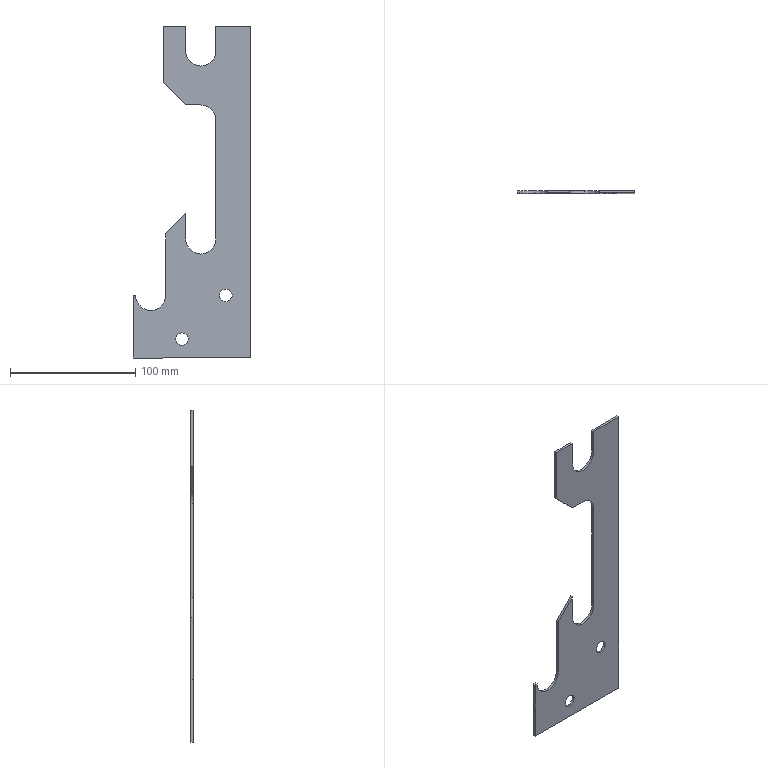Part | SolidWorks | features Extrusion 1 | 1 solid | 28 faces | box 94 x 2 x 265 mm | volume 27822 mm3 | plane 17 | cylinder 11 | commonest cylinder face diameters 24 x7 10 x4
STEP:
#1=CARTESIAN_POINT('',(74.,2.,-5.));
#2=VERTEX_POINT('',#1);
#3=CARTESIAN_POINT('',(74.,2.,5.));
#4=VERTEX_POINT('',#3);
#5=CARTESIAN_POINT('',(74.,2.,0.));
#6=DIRECTION('',(0.,1.,0.));
#7=DIRECTION('',(0.,0.,1.));
#8=AXIS2_PLACEMENT_3D('',#5,#6,#7);
#9=CIRCLE('',#8,5.);
#10=EDGE_CURVE('',#2,#4,#9,.T.);
#11=ORIENTED_EDGE('',*,*,#10,.T.);
#12=CARTESIAN_POINT('',(74.,0.,5.));
#13=VERTEX_POINT('',#12);
#14=CARTESIAN_POINT('',(74.,2.,5.));
#15=DIRECTION('',(0.,-1.,0.));
#16=VECTOR('',#15,1000.);
#17=LINE('',#14,#16);
#18=EDGE_CURVE('',#4,#13,#17,.T.);
#19=ORIENTED_EDGE('',*,*,#18,.T.);
#20=CARTESIAN_POINT('',(74.,0.,-5.));
#21=VERTEX_POINT('',#20);
#22=CARTESIAN_POINT('',(74.,0.,0.));
#23=DIRECTION('',(0.,1.,0.));
#24=DIRECTION('',(0.,0.,1.));
#25=AXIS2_PLACEMENT_3D('',#22,#23,#24);
#26=CIRCLE('',#25,5.);
#27=EDGE_CURVE('',#21,#13,#26,.T.);
#28=ORIENTED_EDGE('',*,*,#27,.F.);
#29=CARTESIAN_POINT('',(74.,2.,-5.));
#30=DIRECTION('',(0.,-1.,0.));
#31=VECTOR('',#30,1000.);
#32=LINE('',#29,#31);
#33=EDGE_CURVE('',#2,#21,#32,.T.);
#34=ORIENTED_EDGE('',*,*,#33,.F.);
#35=EDGE_LOOP('',(#11,#19,#28,#34));
#36=FACE_OUTER_BOUND('',#35,.T.);
#37=CARTESIAN_POINT('',(74.,2.,0.));
#38=DIRECTION('',(0.,-1.,0.));
#39=DIRECTION('',(0.,0.,-1.));
#40=AXIS2_PLACEMENT_3D('',#37,#38,#39);
#41=CYLINDRICAL_SURFACE('',#40,5.);
#42=ADVANCED_FACE('',(#36),#41,.F.);
#43=CARTESIAN_POINT('',(39.,2.,-40.));
#44=VERTEX_POINT('',#43);
#45=CARTESIAN_POINT('',(39.,2.,-30.));
#46=VERTEX_POINT('',#45);
#47=CARTESIAN_POINT('',(39.,2.,-35.));
#48=DIRECTION('',(0.,1.,0.));
#49=DIRECTION('',(0.,0.,1.));
#50=AXIS2_PLACEMENT_3D('',#47,#48,#49);
#51=CIRCLE('',#50,5.);
#52=EDGE_CURVE('',#44,#46,#51,.T.);
#53=ORIENTED_EDGE('',*,*,#52,.T.);
#54=CARTESIAN_POINT('',(39.,0.,-30.));
#55=VERTEX_POINT('',#54);
#56=CARTESIAN_POINT('',(39.,2.,-30.));
#57=DIRECTION('',(0.,-1.,0.));
#58=VECTOR('',#57,1000.);
#59=LINE('',#56,#58);
#60=EDGE_CURVE('',#46,#55,#59,.T.);
#61=ORIENTED_EDGE('',*,*,#60,.T.);
#62=CARTESIAN_POINT('',(39.,0.,-40.));
#63=VERTEX_POINT('',#62);
#64=CARTESIAN_POINT('',(39.,0.,-35.));
#65=DIRECTION('',(0.,1.,0.));
#66=DIRECTION('',(0.,0.,1.));
#67=AXIS2_PLACEMENT_3D('',#64,#65,#66);
#68=CIRCLE('',#67,5.);
#69=EDGE_CURVE('',#63,#55,#68,.T.);
#70=ORIENTED_EDGE('',*,*,#69,.F.);
#71=CARTESIAN_POINT('',(39.,2.,-40.));
#72=DIRECTION('',(0.,-1.,0.));
#73=VECTOR('',#72,1000.);
#74=LINE('',#71,#73);
#75=EDGE_CURVE('',#44,#63,#74,.T.);
#76=ORIENTED_EDGE('',*,*,#75,.F.);
#77=EDGE_LOOP('',(#53,#61,#70,#76));
#78=FACE_OUTER_BOUND('',#77,.T.);
#79=CARTESIAN_POINT('',(39.,2.,-35.));
#80=DIRECTION('',(0.,-1.,0.));
#81=DIRECTION('',(0.,0.,-1.));
#82=AXIS2_PLACEMENT_3D('',#79,#80,#81);
#83=CYLINDRICAL_SURFACE('',#82,5.);
#84=ADVANCED_FACE('',(#78),#83,.F.);
#85=CARTESIAN_POINT('',(54.,2.,183.));
#86=VERTEX_POINT('',#85);
#87=CARTESIAN_POINT('',(66.,2.,195.));
#88=VERTEX_POINT('',#87);
#89=CARTESIAN_POINT('',(54.,2.,195.));
#90=DIRECTION('',(0.,-1.,0.));
#91=DIRECTION('',(0.,0.,1.));
#92=AXIS2_PLACEMENT_3D('',#89,#90,#91);
#93=CIRCLE('',#92,12.);
#94=EDGE_CURVE('',#86,#88,#93,.T.);
#95=ORIENTED_EDGE('',*,*,#94,.F.);
#96=CARTESIAN_POINT('',(54.,0.,183.));
#97=VERTEX_POINT('',#96);
#98=CARTESIAN_POINT('',(54.,2.,183.));
#99=DIRECTION('',(0.,-1.,0.));
#100=VECTOR('',#99,1000.);
#101=LINE('',#98,#100);
#102=EDGE_CURVE('',#86,#97,#101,.T.);
#103=ORIENTED_EDGE('',*,*,#102,.T.);
#104=CARTESIAN_POINT('',(66.,0.,195.));
#105=VERTEX_POINT('',#104);
#106=CARTESIAN_POINT('',(54.,0.,195.));
#107=DIRECTION('',(0.,-1.,0.));
#108=DIRECTION('',(0.,0.,1.));
#109=AXIS2_PLACEMENT_3D('',#106,#107,#108);
#110=CIRCLE('',#109,12.);
#111=EDGE_CURVE('',#97,#105,#110,.T.);
#112=ORIENTED_EDGE('',*,*,#111,.T.);
#113=CARTESIAN_POINT('',(66.,2.,195.));
#114=DIRECTION('',(0.,-1.,0.));
#115=VECTOR('',#114,1000.);
#116=LINE('',#113,#115);
#117=EDGE_CURVE('',#88,#105,#116,.T.);
#118=ORIENTED_EDGE('',*,*,#117,.F.);
#119=EDGE_LOOP('',(#95,#103,#112,#118));
#120=FACE_OUTER_BOUND('',#119,.T.);
#121=CARTESIAN_POINT('',(54.,2.,195.));
#122=DIRECTION('',(0.,-1.,0.));
#123=DIRECTION('',(0.,0.,-1.));
#124=AXIS2_PLACEMENT_3D('',#121,#122,#123);
#125=CYLINDRICAL_SURFACE('',#124,12.);
#126=ADVANCED_FACE('',(#120),#125,.F.);
#127=CARTESIAN_POINT('',(54.,2.,33.));
#128=VERTEX_POINT('',#127);
#129=CARTESIAN_POINT('',(66.,2.,45.));
#130=VERTEX_POINT('',#129);
#131=CARTESIAN_POINT('',(54.,2.,45.));
#132=DIRECTION('',(0.,-1.,0.));
#133=DIRECTION('',(0.,0.,1.));
#134=AXIS2_PLACEMENT_3D('',#131,#132,#133);
#135=CIRCLE('',#134,12.);
#136=EDGE_CURVE('',#128,#130,#135,.T.);
#137=ORIENTED_EDGE('',*,*,#136,.F.);
#138=CARTESIAN_POINT('',(54.,0.,33.));
#139=VERTEX_POINT('',#138);
#140=CARTESIAN_POINT('',(54.,2.,33.));
#141=DIRECTION('',(0.,-1.,0.));
#142=VECTOR('',#141,1000.);
#143=LINE('',#140,#142);
#144=EDGE_CURVE('',#128,#139,#143,.T.);
#145=ORIENTED_EDGE('',*,*,#144,.T.);
#146=CARTESIAN_POINT('',(66.,0.,45.));
#147=VERTEX_POINT('',#146);
#148=CARTESIAN_POINT('',(54.,0.,45.));
#149=DIRECTION('',(0.,-1.,0.));
#150=DIRECTION('',(0.,0.,1.));
#151=AXIS2_PLACEMENT_3D('',#148,#149,#150);
#152=CIRCLE('',#151,12.);
#153=EDGE_CURVE('',#139,#147,#152,.T.);
#154=ORIENTED_EDGE('',*,*,#153,.T.);
#155=CARTESIAN_POINT('',(66.,2.,45.));
#156=DIRECTION('',(0.,-1.,0.));
#157=VECTOR('',#156,1000.);
#158=LINE('',#155,#157);
#159=EDGE_CURVE('',#130,#147,#158,.T.);
#160=ORIENTED_EDGE('',*,*,#159,.F.);
#161=EDGE_LOOP('',(#137,#145,#154,#160));
#162=FACE_OUTER_BOUND('',#161,.T.);
#163=CARTESIAN_POINT('',(54.,2.,45.));
#164=DIRECTION('',(0.,-1.,0.));
#165=DIRECTION('',(0.,0.,-1.));
#166=AXIS2_PLACEMENT_3D('',#163,#164,#165);
#167=CYLINDRICAL_SURFACE('',#166,12.);
#168=ADVANCED_FACE('',(#162),#167,.F.);
#169=CARTESIAN_POINT('',(14.,2.,-12.));
#170=VERTEX_POINT('',#169);
#171=CARTESIAN_POINT('',(26.,2.,0.));
#172=VERTEX_POINT('',#171);
#173=CARTESIAN_POINT('',(14.,2.,0.));
#174=DIRECTION('',(0.,-1.,0.));
#175=DIRECTION('',(0.,0.,1.));
#176=AXIS2_PLACEMENT_3D('',#173,#174,#175);
#177=CIRCLE('',#176,12.);
#178=EDGE_CURVE('',#170,#172,#177,.T.);
#179=ORIENTED_EDGE('',*,*,#178,.F.);
#180=CARTESIAN_POINT('',(14.,0.,-12.));
#181=VERTEX_POINT('',#180);
#182=CARTESIAN_POINT('',(14.,2.,-12.));
#183=DIRECTION('',(0.,-1.,0.));
#184=VECTOR('',#183,1000.);
#185=LINE('',#182,#184);
#186=EDGE_CURVE('',#170,#181,#185,.T.);
#187=ORIENTED_EDGE('',*,*,#186,.T.);
#188=CARTESIAN_POINT('',(26.,0.,0.));
#189=VERTEX_POINT('',#188);
#190=CARTESIAN_POINT('',(14.,0.,0.));
#191=DIRECTION('',(0.,-1.,0.));
#192=DIRECTION('',(0.,0.,1.));
#193=AXIS2_PLACEMENT_3D('',#190,#191,#192);
#194=CIRCLE('',#193,12.);
#195=EDGE_CURVE('',#181,#189,#194,.T.);
#196=ORIENTED_EDGE('',*,*,#195,.T.);
#197=CARTESIAN_POINT('',(26.,2.,0.));
#198=DIRECTION('',(0.,-1.,0.));
#199=VECTOR('',#198,1000.);
#200=LINE('',#197,#199);
#201=EDGE_CURVE('',#172,#189,#200,.T.);
#202=ORIENTED_EDGE('',*,*,#201,.F.);
#203=EDGE_LOOP('',(#179,#187,#196,#202));
#204=FACE_OUTER_BOUND('',#203,.T.);
#205=CARTESIAN_POINT('',(14.,2.,0.));
#206=DIRECTION('',(0.,-1.,0.));
#207=DIRECTION('',(0.,0.,-1.));
#208=AXIS2_PLACEMENT_3D('',#205,#206,#207);
#209=CYLINDRICAL_SURFACE('',#208,12.);
#210=ADVANCED_FACE('',(#204),#209,.F.);
#211=ORIENTED_EDGE('',*,*,#52,.F.);
#212=CARTESIAN_POINT('',(39.,2.,-35.));
#213=DIRECTION('',(0.,1.,0.));
#214=DIRECTION('',(0.,0.,1.));
#215=AXIS2_PLACEMENT_3D('',#212,#213,#214);
#216=CIRCLE('',#215,5.);
#217=EDGE_CURVE('',#46,#44,#216,.T.);
#218=ORIENTED_EDGE('',*,*,#217,.F.);
#219=EDGE_LOOP('',(#211,#218));
#220=FACE_BOUND('',#219,.T.);
#221=CARTESIAN_POINT('',(0.,2.,0.));
#222=VERTEX_POINT('',#221);
#223=CARTESIAN_POINT('',(2.,2.,0.));
#224=VERTEX_POINT('',#223);
#225=CARTESIAN_POINT('',(0.,2.,0.));
#226=DIRECTION('',(1.,0.,0.));
#227=VECTOR('',#226,1000.);
#228=LINE('',#225,#227);
#229=EDGE_CURVE('',#222,#224,#228,.T.);
#230=ORIENTED_EDGE('',*,*,#229,.T.);
#231=CARTESIAN_POINT('',(14.,2.,0.));
#232=DIRECTION('',(0.,-1.,0.));
#233=DIRECTION('',(0.,0.,1.));
#234=AXIS2_PLACEMENT_3D('',#231,#232,#233);
#235=CIRCLE('',#234,12.);
#236=EDGE_CURVE('',#224,#170,#235,.T.);
#237=ORIENTED_EDGE('',*,*,#236,.T.);
#238=ORIENTED_EDGE('',*,*,#178,.T.);
#239=CARTESIAN_POINT('',(26.,2.,49.));
#240=VERTEX_POINT('',#239);
#241=CARTESIAN_POINT('',(26.,2.,49.));
#242=DIRECTION('',(0.,0.,1.));
#243=VECTOR('',#242,1000.);
#244=LINE('',#241,#243);
#245=EDGE_CURVE('',#172,#240,#244,.T.);
#246=ORIENTED_EDGE('',*,*,#245,.T.);
#247=CARTESIAN_POINT('',(42.,2.,65.));
#248=VERTEX_POINT('',#247);
#249=CARTESIAN_POINT('',(42.,2.,65.));
#250=DIRECTION('',(0.7071,0.,0.7071));
#251=VECTOR('',#250,1000.);
#252=LINE('',#249,#251);
#253=EDGE_CURVE('',#240,#248,#252,.T.);
#254=ORIENTED_EDGE('',*,*,#253,.T.);
#255=CARTESIAN_POINT('',(42.,2.,45.));
#256=VERTEX_POINT('',#255);
#257=CARTESIAN_POINT('',(42.,2.,45.));
#258=DIRECTION('',(0.,0.,-1.));
#259=VECTOR('',#258,1000.);
#260=LINE('',#257,#259);
#261=EDGE_CURVE('',#248,#256,#260,.T.);
#262=ORIENTED_EDGE('',*,*,#261,.T.);
#263=CARTESIAN_POINT('',(54.,2.,45.));
#264=DIRECTION('',(0.,-1.,0.));
#265=DIRECTION('',(0.,0.,1.));
#266=AXIS2_PLACEMENT_3D('',#263,#264,#265);
#267=CIRCLE('',#266,12.);
#268=EDGE_CURVE('',#256,#128,#267,.T.);
#269=ORIENTED_EDGE('',*,*,#268,.T.);
#270=ORIENTED_EDGE('',*,*,#136,.T.);
#271=CARTESIAN_POINT('',(66.,2.,140.));
#272=VERTEX_POINT('',#271);
#273=CARTESIAN_POINT('',(66.,2.,45.));
#274=DIRECTION('',(0.,0.,1.));
#275=VECTOR('',#274,1000.);
#276=LINE('',#273,#275);
#277=EDGE_CURVE('',#130,#272,#276,.T.);
#278=ORIENTED_EDGE('',*,*,#277,.T.);
#279=CARTESIAN_POINT('',(54.,2.,152.));
#280=VERTEX_POINT('',#279);
#281=CARTESIAN_POINT('',(54.,2.,140.));
#282=DIRECTION('',(0.,-1.,0.));
#283=DIRECTION('',(0.,0.,-1.));
#284=AXIS2_PLACEMENT_3D('',#281,#282,#283);
#285=CIRCLE('',#284,12.);
#286=EDGE_CURVE('',#272,#280,#285,.T.);
#287=ORIENTED_EDGE('',*,*,#286,.T.);
#288=CARTESIAN_POINT('',(42.,2.,152.));
#289=VERTEX_POINT('',#288);
#290=CARTESIAN_POINT('',(54.,2.,152.));
#291=DIRECTION('',(-1.,0.,0.));
#292=VECTOR('',#291,1000.);
#293=LINE('',#290,#292);
#294=EDGE_CURVE('',#280,#289,#293,.T.);
#295=ORIENTED_EDGE('',*,*,#294,.T.);
#296=CARTESIAN_POINT('',(24.,2.,170.));
#297=VERTEX_POINT('',#296);
#298=CARTESIAN_POINT('',(42.,2.,152.));
#299=DIRECTION('',(-0.7071,0.,0.7071));
#300=VECTOR('',#299,1000.);
#301=LINE('',#298,#300);
#302=EDGE_CURVE('',#289,#297,#301,.T.);
#303=ORIENTED_EDGE('',*,*,#302,.T.);
#304=CARTESIAN_POINT('',(24.,2.,215.));
#305=VERTEX_POINT('',#304);
#306=CARTESIAN_POINT('',(24.,2.,170.));
#307=DIRECTION('',(0.,0.,1.));
#308=VECTOR('',#307,1000.);
#309=LINE('',#306,#308);
#310=EDGE_CURVE('',#297,#305,#309,.T.);
#311=ORIENTED_EDGE('',*,*,#310,.T.);
#312=CARTESIAN_POINT('',(42.,2.,215.));
#313=VERTEX_POINT('',#312);
#314=CARTESIAN_POINT('',(24.,2.,215.));
#315=DIRECTION('',(1.,0.,0.));
#316=VECTOR('',#315,1000.);
#317=LINE('',#314,#316);
#318=EDGE_CURVE('',#305,#313,#317,.T.);
#319=ORIENTED_EDGE('',*,*,#318,.T.);
#320=CARTESIAN_POINT('',(42.,2.,195.));
#321=VERTEX_POINT('',#320);
#322=CARTESIAN_POINT('',(42.,2.,215.));
#323=DIRECTION('',(0.,0.,-1.));
#324=VECTOR('',#323,1000.);
#325=LINE('',#322,#324);
#326=EDGE_CURVE('',#313,#321,#325,.T.);
#327=ORIENTED_EDGE('',*,*,#326,.T.);
#328=CARTESIAN_POINT('',(54.,2.,195.));
#329=DIRECTION('',(0.,-1.,0.));
#330=DIRECTION('',(0.,0.,1.));
#331=AXIS2_PLACEMENT_3D('',#328,#329,#330);
#332=CIRCLE('',#331,12.);
#333=EDGE_CURVE('',#321,#86,#332,.T.);
#334=ORIENTED_EDGE('',*,*,#333,.T.);
#335=ORIENTED_EDGE('',*,*,#94,.T.);
#336=CARTESIAN_POINT('',(66.,2.,215.));
#337=VERTEX_POINT('',#336);
#338=CARTESIAN_POINT('',(66.,2.,195.));
#339=DIRECTION('',(0.,0.,1.));
#340=VECTOR('',#339,1000.);
#341=LINE('',#338,#340);
#342=EDGE_CURVE('',#88,#337,#341,.T.);
#343=ORIENTED_EDGE('',*,*,#342,.T.);
#344=CARTESIAN_POINT('',(94.,2.,215.));
#345=VERTEX_POINT('',#344);
#346=CARTESIAN_POINT('',(94.,2.,215.));
#347=DIRECTION('',(1.,0.,0.));
#348=VECTOR('',#347,1000.);
#349=LINE('',#346,#348);
#350=EDGE_CURVE('',#337,#345,#349,.T.);
#351=ORIENTED_EDGE('',*,*,#350,.T.);
#352=CARTESIAN_POINT('',(94.,2.,-50.));
#353=VERTEX_POINT('',#352);
#354=CARTESIAN_POINT('',(94.,2.,-50.));
#355=DIRECTION('',(0.,0.,-1.));
#356=VECTOR('',#355,1000.);
#357=LINE('',#354,#356);
#358=EDGE_CURVE('',#345,#353,#357,.T.);
#359=ORIENTED_EDGE('',*,*,#358,.T.);
#360=CARTESIAN_POINT('',(0.,2.,-50.));
#361=VERTEX_POINT('',#360);
#362=CARTESIAN_POINT('',(0.,2.,-50.));
#363=DIRECTION('',(-1.,0.,0.));
#364=VECTOR('',#363,1000.);
#365=LINE('',#362,#364);
#366=EDGE_CURVE('',#353,#361,#365,.T.);
#367=ORIENTED_EDGE('',*,*,#366,.T.);
#368=CARTESIAN_POINT('',(0.,2.,0.));
#369=DIRECTION('',(0.,0.,1.));
#370=VECTOR('',#369,1000.);
#371=LINE('',#368,#370);
#372=EDGE_CURVE('',#361,#222,#371,.T.);
#373=ORIENTED_EDGE('',*,*,#372,.T.);
#374=EDGE_LOOP('',(#230,#237,#238,#246,#254,#262,#269,#270,#278,#287,#295,#303,#311,#319,#327,#334,#335,#343,#351,#359,#367,#373));
#375=FACE_OUTER_BOUND('',#374,.T.);
#376=ORIENTED_EDGE('',*,*,#10,.F.);
#377=CARTESIAN_POINT('',(74.,2.,0.));
#378=DIRECTION('',(0.,1.,0.));
#379=DIRECTION('',(0.,0.,1.));
#380=AXIS2_PLACEMENT_3D('',#377,#378,#379);
#381=CIRCLE('',#380,5.);
#382=EDGE_CURVE('',#4,#2,#381,.T.);
#383=ORIENTED_EDGE('',*,*,#382,.F.);
#384=EDGE_LOOP('',(#376,#383));
#385=FACE_BOUND('',#384,.T.);
#386=CARTESIAN_POINT('',(14.,2.,0.));
#387=DIRECTION('',(0.,1.,0.));
#388=DIRECTION('',(0.,0.,1.));
#389=AXIS2_PLACEMENT_3D('',#386,#387,#388);
#390=PLANE('',#389);
#391=ADVANCED_FACE('',(#220,#375,#385),#390,.T.);
#392=CARTESIAN_POINT('',(0.,0.,0.));
#393=VERTEX_POINT('',#392);
#394=CARTESIAN_POINT('',(2.,0.,0.));
#395=VERTEX_POINT('',#394);
#396=CARTESIAN_POINT('',(0.,0.,0.));
#397=DIRECTION('',(1.,0.,0.));
#398=VECTOR('',#397,1000.);
#399=LINE('',#396,#398);
#400=EDGE_CURVE('',#393,#395,#399,.T.);
#401=ORIENTED_EDGE('',*,*,#400,.F.);
#402=CARTESIAN_POINT('',(0.,0.,-50.));
#403=VERTEX_POINT('',#402);
#404=CARTESIAN_POINT('',(0.,0.,0.));
#405=DIRECTION('',(0.,0.,1.));
#406=VECTOR('',#405,1000.);
#407=LINE('',#404,#406);
#408=EDGE_CURVE('',#403,#393,#407,.T.);
#409=ORIENTED_EDGE('',*,*,#408,.F.);
#410=CARTESIAN_POINT('',(94.,0.,-50.));
#411=VERTEX_POINT('',#410);
#412=CARTESIAN_POINT('',(0.,0.,-50.));
#413=DIRECTION('',(-1.,0.,0.));
#414=VECTOR('',#413,1000.);
#415=LINE('',#412,#414);
#416=EDGE_CURVE('',#411,#403,#415,.T.);
#417=ORIENTED_EDGE('',*,*,#416,.F.);
#418=CARTESIAN_POINT('',(94.,0.,215.));
#419=VERTEX_POINT('',#418);
#420=CARTESIAN_POINT('',(94.,0.,-50.));
#421=DIRECTION('',(0.,0.,-1.));
#422=VECTOR('',#421,1000.);
#423=LINE('',#420,#422);
#424=EDGE_CURVE('',#419,#411,#423,.T.);
#425=ORIENTED_EDGE('',*,*,#424,.F.);
#426=CARTESIAN_POINT('',(66.,0.,215.));
#427=VERTEX_POINT('',#426);
#428=CARTESIAN_POINT('',(94.,0.,215.));
#429=DIRECTION('',(1.,0.,0.));
#430=VECTOR('',#429,1000.);
#431=LINE('',#428,#430);
#432=EDGE_CURVE('',#427,#419,#431,.T.);
#433=ORIENTED_EDGE('',*,*,#432,.F.);
#434=CARTESIAN_POINT('',(66.,0.,195.));
#435=DIRECTION('',(0.,0.,1.));
#436=VECTOR('',#435,1000.);
#437=LINE('',#434,#436);
#438=EDGE_CURVE('',#105,#427,#437,.T.);
#439=ORIENTED_EDGE('',*,*,#438,.F.);
#440=ORIENTED_EDGE('',*,*,#111,.F.);
#441=CARTESIAN_POINT('',(42.,0.,195.));
#442=VERTEX_POINT('',#441);
#443=CARTESIAN_POINT('',(54.,0.,195.));
#444=DIRECTION('',(0.,-1.,0.));
#445=DIRECTION('',(0.,0.,1.));
#446=AXIS2_PLACEMENT_3D('',#443,#444,#445);
#447=CIRCLE('',#446,12.);
#448=EDGE_CURVE('',#442,#97,#447,.T.);
#449=ORIENTED_EDGE('',*,*,#448,.F.);
#450=CARTESIAN_POINT('',(42.,0.,215.));
#451=VERTEX_POINT('',#450);
#452=CARTESIAN_POINT('',(42.,0.,215.));
#453=DIRECTION('',(0.,0.,-1.));
#454=VECTOR('',#453,1000.);
#455=LINE('',#452,#454);
#456=EDGE_CURVE('',#451,#442,#455,.T.);
#457=ORIENTED_EDGE('',*,*,#456,.F.);
#458=CARTESIAN_POINT('',(24.,0.,215.));
#459=VERTEX_POINT('',#458);
#460=CARTESIAN_POINT('',(24.,0.,215.));
#461=DIRECTION('',(1.,0.,0.));
#462=VECTOR('',#461,1000.);
#463=LINE('',#460,#462);
#464=EDGE_CURVE('',#459,#451,#463,.T.);
#465=ORIENTED_EDGE('',*,*,#464,.F.);
#466=CARTESIAN_POINT('',(24.,0.,170.));
#467=VERTEX_POINT('',#466);
#468=CARTESIAN_POINT('',(24.,0.,170.));
#469=DIRECTION('',(0.,0.,1.));
#470=VECTOR('',#469,1000.);
#471=LINE('',#468,#470);
#472=EDGE_CURVE('',#467,#459,#471,.T.);
#473=ORIENTED_EDGE('',*,*,#472,.F.);
#474=CARTESIAN_POINT('',(42.,0.,152.));
#475=VERTEX_POINT('',#474);
#476=CARTESIAN_POINT('',(42.,0.,152.));
#477=DIRECTION('',(-0.7071,0.,0.7071));
#478=VECTOR('',#477,1000.);
#479=LINE('',#476,#478);
#480=EDGE_CURVE('',#475,#467,#479,.T.);
#481=ORIENTED_EDGE('',*,*,#480,.F.);
#482=CARTESIAN_POINT('',(54.,0.,152.));
#483=VERTEX_POINT('',#482);
#484=CARTESIAN_POINT('',(54.,0.,152.));
#485=DIRECTION('',(-1.,0.,0.));
#486=VECTOR('',#485,1000.);
#487=LINE('',#484,#486);
#488=EDGE_CURVE('',#483,#475,#487,.T.);
#489=ORIENTED_EDGE('',*,*,#488,.F.);
#490=CARTESIAN_POINT('',(66.,0.,140.));
#491=VERTEX_POINT('',#490);
#492=CARTESIAN_POINT('',(54.,0.,140.));
#493=DIRECTION('',(0.,-1.,0.));
#494=DIRECTION('',(0.,0.,-1.));
#495=AXIS2_PLACEMENT_3D('',#492,#493,#494);
#496=CIRCLE('',#495,12.);
#497=EDGE_CURVE('',#491,#483,#496,.T.);
#498=ORIENTED_EDGE('',*,*,#497,.F.);
#499=CARTESIAN_POINT('',(66.,0.,45.));
#500=DIRECTION('',(0.,0.,1.));
#501=VECTOR('',#500,1000.);
#502=LINE('',#499,#501);
#503=EDGE_CURVE('',#147,#491,#502,.T.);
#504=ORIENTED_EDGE('',*,*,#503,.F.);
#505=ORIENTED_EDGE('',*,*,#153,.F.);
#506=CARTESIAN_POINT('',(42.,0.,45.));
#507=VERTEX_POINT('',#506);
#508=CARTESIAN_POINT('',(54.,0.,45.));
#509=DIRECTION('',(0.,-1.,0.));
#510=DIRECTION('',(0.,0.,1.));
#511=AXIS2_PLACEMENT_3D('',#508,#509,#510);
#512=CIRCLE('',#511,12.);
#513=EDGE_CURVE('',#507,#139,#512,.T.);
#514=ORIENTED_EDGE('',*,*,#513,.F.);
#515=CARTESIAN_POINT('',(42.,0.,65.));
#516=VERTEX_POINT('',#515);
#517=CARTESIAN_POINT('',(42.,0.,45.));
#518=DIRECTION('',(0.,0.,-1.));
#519=VECTOR('',#518,1000.);
#520=LINE('',#517,#519);
#521=EDGE_CURVE('',#516,#507,#520,.T.);
#522=ORIENTED_EDGE('',*,*,#521,.F.);
#523=CARTESIAN_POINT('',(26.,0.,49.));
#524=VERTEX_POINT('',#523);
#525=CARTESIAN_POINT('',(42.,0.,65.));
#526=DIRECTION('',(0.7071,0.,0.7071));
#527=VECTOR('',#526,1000.);
#528=LINE('',#525,#527);
#529=EDGE_CURVE('',#524,#516,#528,.T.);
#530=ORIENTED_EDGE('',*,*,#529,.F.);
#531=CARTESIAN_POINT('',(26.,0.,49.));
#532=DIRECTION('',(0.,0.,1.));
#533=VECTOR('',#532,1000.);
#534=LINE('',#531,#533);
#535=EDGE_CURVE('',#189,#524,#534,.T.);
#536=ORIENTED_EDGE('',*,*,#535,.F.);
#537=ORIENTED_EDGE('',*,*,#195,.F.);
#538=CARTESIAN_POINT('',(14.,0.,0.));
#539=DIRECTION('',(0.,-1.,0.));
#540=DIRECTION('',(0.,0.,1.));
#541=AXIS2_PLACEMENT_3D('',#538,#539,#540);
#542=CIRCLE('',#541,12.);
#543=EDGE_CURVE('',#395,#181,#542,.T.);
#544=ORIENTED_EDGE('',*,*,#543,.F.);
#545=EDGE_LOOP('',(#401,#409,#417,#425,#433,#439,#440,#449,#457,#465,#473,#481,#489,#498,#504,#505,#514,#522,#530,#536,#537,#544));
#546=FACE_OUTER_BOUND('',#545,.T.);
#547=ORIENTED_EDGE('',*,*,#69,.T.);
#548=CARTESIAN_POINT('',(39.,0.,-35.));
#549=DIRECTION('',(0.,1.,0.));
#550=DIRECTION('',(0.,0.,1.));
#551=AXIS2_PLACEMENT_3D('',#548,#549,#550);
#552=CIRCLE('',#551,5.);
#553=EDGE_CURVE('',#55,#63,#552,.T.);
#554=ORIENTED_EDGE('',*,*,#553,.T.);
#555=EDGE_LOOP('',(#547,#554));
#556=FACE_BOUND('',#555,.T.);
#557=ORIENTED_EDGE('',*,*,#27,.T.);
#558=CARTESIAN_POINT('',(74.,0.,0.));
#559=DIRECTION('',(0.,1.,0.));
#560=DIRECTION('',(0.,0.,1.));
#561=AXIS2_PLACEMENT_3D('',#558,#559,#560);
#562=CIRCLE('',#561,5.);
#563=EDGE_CURVE('',#13,#21,#562,.T.);
#564=ORIENTED_EDGE('',*,*,#563,.T.);
#565=EDGE_LOOP('',(#557,#564));
#566=FACE_BOUND('',#565,.T.);
#567=CARTESIAN_POINT('',(14.,0.,0.));
#568=DIRECTION('',(0.,1.,0.));
#569=DIRECTION('',(0.,0.,1.));
#570=AXIS2_PLACEMENT_3D('',#567,#568,#569);
#571=PLANE('',#570);
#572=ADVANCED_FACE('',(#546,#556,#566),#571,.F.);
#573=ORIENTED_EDGE('',*,*,#400,.T.);
#574=CARTESIAN_POINT('',(2.,2.,0.));
#575=DIRECTION('',(0.,-1.,0.));
#576=VECTOR('',#575,1000.);
#577=LINE('',#574,#576);
#578=EDGE_CURVE('',#224,#395,#577,.T.);
#579=ORIENTED_EDGE('',*,*,#578,.F.);
#580=ORIENTED_EDGE('',*,*,#229,.F.);
#581=CARTESIAN_POINT('',(0.,2.,0.));
#582=DIRECTION('',(0.,-1.,0.));
#583=VECTOR('',#582,1000.);
#584=LINE('',#581,#583);
#585=EDGE_CURVE('',#222,#393,#584,.T.);
#586=ORIENTED_EDGE('',*,*,#585,.T.);
#587=EDGE_LOOP('',(#573,#579,#580,#586));
#588=FACE_OUTER_BOUND('',#587,.T.);
#589=CARTESIAN_POINT('',(0.,2.,0.));
#590=DIRECTION('',(0.,0.,-1.));
#591=DIRECTION('',(-1.,0.,0.));
#592=AXIS2_PLACEMENT_3D('',#589,#590,#591);
#593=PLANE('',#592);
#594=ADVANCED_FACE('',(#588),#593,.F.);
#595=ORIENTED_EDGE('',*,*,#186,.F.);
#596=ORIENTED_EDGE('',*,*,#236,.F.);
#597=ORIENTED_EDGE('',*,*,#578,.T.);
#598=ORIENTED_EDGE('',*,*,#543,.T.);
#599=EDGE_LOOP('',(#595,#596,#597,#598));
#600=FACE_OUTER_BOUND('',#599,.T.);
#601=CARTESIAN_POINT('',(14.,2.,0.));
#602=DIRECTION('',(0.,-1.,0.));
#603=DIRECTION('',(0.,0.,-1.));
#604=AXIS2_PLACEMENT_3D('',#601,#602,#603);
#605=CYLINDRICAL_SURFACE('',#604,12.);
#606=ADVANCED_FACE('',(#600),#605,.F.);
#607=ORIENTED_EDGE('',*,*,#535,.T.);
#608=CARTESIAN_POINT('',(26.,2.,49.));
#609=DIRECTION('',(0.,-1.,0.));
#610=VECTOR('',#609,1000.);
#611=LINE('',#608,#610);
#612=EDGE_CURVE('',#240,#524,#611,.T.);
#613=ORIENTED_EDGE('',*,*,#612,.F.);
#614=ORIENTED_EDGE('',*,*,#245,.F.);
#615=ORIENTED_EDGE('',*,*,#201,.T.);
#616=EDGE_LOOP('',(#607,#613,#614,#615));
#617=FACE_OUTER_BOUND('',#616,.T.);
#618=CARTESIAN_POINT('',(26.,2.,49.));
#619=DIRECTION('',(1.,0.,0.));
#620=DIRECTION('',(0.,0.,-1.));
#621=AXIS2_PLACEMENT_3D('',#618,#619,#620);
#622=PLANE('',#621);
#623=ADVANCED_FACE('',(#617),#622,.F.);
#624=ORIENTED_EDGE('',*,*,#529,.T.);
#625=CARTESIAN_POINT('',(42.,2.,65.));
#626=DIRECTION('',(0.,-1.,0.));
#627=VECTOR('',#626,1000.);
#628=LINE('',#625,#627);
#629=EDGE_CURVE('',#248,#516,#628,.T.);
#630=ORIENTED_EDGE('',*,*,#629,.F.);
#631=ORIENTED_EDGE('',*,*,#253,.F.);
#632=ORIENTED_EDGE('',*,*,#612,.T.);
#633=EDGE_LOOP('',(#624,#630,#631,#632));
#634=FACE_OUTER_BOUND('',#633,.T.);
#635=CARTESIAN_POINT('',(42.,2.,65.));
#636=DIRECTION('',(0.7071,0.,-0.7071));
#637=DIRECTION('',(-0.7071,0.,-0.7071));
#638=AXIS2_PLACEMENT_3D('',#635,#636,#637);
#639=PLANE('',#638);
#640=ADVANCED_FACE('',(#634),#639,.F.);
#641=ORIENTED_EDGE('',*,*,#521,.T.);
#642=CARTESIAN_POINT('',(42.,2.,45.));
#643=DIRECTION('',(0.,-1.,0.));
#644=VECTOR('',#643,1000.);
#645=LINE('',#642,#644);
#646=EDGE_CURVE('',#256,#507,#645,.T.);
#647=ORIENTED_EDGE('',*,*,#646,.F.);
#648=ORIENTED_EDGE('',*,*,#261,.F.);
#649=ORIENTED_EDGE('',*,*,#629,.T.);
#650=EDGE_LOOP('',(#641,#647,#648,#649));
#651=FACE_OUTER_BOUND('',#650,.T.);
#652=CARTESIAN_POINT('',(42.,2.,45.));
#653=DIRECTION('',(-1.,0.,0.));
#654=DIRECTION('',(0.,0.,1.));
#655=AXIS2_PLACEMENT_3D('',#652,#653,#654);
#656=PLANE('',#655);
#657=ADVANCED_FACE('',(#651),#656,.F.);
#658=ORIENTED_EDGE('',*,*,#144,.F.);
#659=ORIENTED_EDGE('',*,*,#268,.F.);
#660=ORIENTED_EDGE('',*,*,#646,.T.);
#661=ORIENTED_EDGE('',*,*,#513,.T.);
#662=EDGE_LOOP('',(#658,#659,#660,#661));
#663=FACE_OUTER_BOUND('',#662,.T.);
#664=CARTESIAN_POINT('',(54.,2.,45.));
#665=DIRECTION('',(0.,-1.,0.));
#666=DIRECTION('',(0.,0.,-1.));
#667=AXIS2_PLACEMENT_3D('',#664,#665,#666);
#668=CYLINDRICAL_SURFACE('',#667,12.);
#669=ADVANCED_FACE('',(#663),#668,.F.);
#670=ORIENTED_EDGE('',*,*,#503,.T.);
#671=CARTESIAN_POINT('',(66.,2.,140.));
#672=DIRECTION('',(0.,-1.,0.));
#673=VECTOR('',#672,1000.);
#674=LINE('',#671,#673);
#675=EDGE_CURVE('',#272,#491,#674,.T.);
#676=ORIENTED_EDGE('',*,*,#675,.F.);
#677=ORIENTED_EDGE('',*,*,#277,.F.);
#678=ORIENTED_EDGE('',*,*,#159,.T.);
#679=EDGE_LOOP('',(#670,#676,#677,#678));
#680=FACE_OUTER_BOUND('',#679,.T.);
#681=CARTESIAN_POINT('',(66.,2.,45.));
#682=DIRECTION('',(1.,0.,0.));
#683=DIRECTION('',(0.,0.,-1.));
#684=AXIS2_PLACEMENT_3D('',#681,#682,#683);
#685=PLANE('',#684);
#686=ADVANCED_FACE('',(#680),#685,.F.);
#687=ORIENTED_EDGE('',*,*,#497,.T.);
#688=CARTESIAN_POINT('',(54.,2.,152.));
#689=DIRECTION('',(0.,-1.,0.));
#690=VECTOR('',#689,1000.);
#691=LINE('',#688,#690);
#692=EDGE_CURVE('',#280,#483,#691,.T.);
#693=ORIENTED_EDGE('',*,*,#692,.F.);
#694=ORIENTED_EDGE('',*,*,#286,.F.);
#695=ORIENTED_EDGE('',*,*,#675,.T.);
#696=EDGE_LOOP('',(#687,#693,#694,#695));
#697=FACE_OUTER_BOUND('',#696,.T.);
#698=CARTESIAN_POINT('',(54.,2.,140.));
#699=DIRECTION('',(0.,-1.,0.));
#700=DIRECTION('',(0.,0.,-1.));
#701=AXIS2_PLACEMENT_3D('',#698,#699,#700);
#702=CYLINDRICAL_SURFACE('',#701,12.);
#703=ADVANCED_FACE('',(#697),#702,.F.);
#704=ORIENTED_EDGE('',*,*,#488,.T.);
#705=CARTESIAN_POINT('',(42.,2.,152.));
#706=DIRECTION('',(0.,-1.,0.));
#707=VECTOR('',#706,1000.);
#708=LINE('',#705,#707);
#709=EDGE_CURVE('',#289,#475,#708,.T.);
#710=ORIENTED_EDGE('',*,*,#709,.F.);
#711=ORIENTED_EDGE('',*,*,#294,.F.);
#712=ORIENTED_EDGE('',*,*,#692,.T.);
#713=EDGE_LOOP('',(#704,#710,#711,#712));
#714=FACE_OUTER_BOUND('',#713,.T.);
#715=CARTESIAN_POINT('',(54.,2.,152.));
#716=DIRECTION('',(0.,0.,1.));
#717=DIRECTION('',(1.,0.,0.));
#718=AXIS2_PLACEMENT_3D('',#715,#716,#717);
#719=PLANE('',#718);
#720=ADVANCED_FACE('',(#714),#719,.F.);
#721=ORIENTED_EDGE('',*,*,#480,.T.);
#722=CARTESIAN_POINT('',(24.,2.,170.));
#723=DIRECTION('',(0.,-1.,0.));
#724=VECTOR('',#723,1000.);
#725=LINE('',#722,#724);
#726=EDGE_CURVE('',#297,#467,#725,.T.);
#727=ORIENTED_EDGE('',*,*,#726,.F.);
#728=ORIENTED_EDGE('',*,*,#302,.F.);
#729=ORIENTED_EDGE('',*,*,#709,.T.);
#730=EDGE_LOOP('',(#721,#727,#728,#729));
#731=FACE_OUTER_BOUND('',#730,.T.);
#732=CARTESIAN_POINT('',(42.,2.,152.));
#733=DIRECTION('',(0.7071,0.,0.7071));
#734=DIRECTION('',(0.7071,0.,-0.7071));
#735=AXIS2_PLACEMENT_3D('',#732,#733,#734);
#736=PLANE('',#735);
#737=ADVANCED_FACE('',(#731),#736,.F.);
#738=ORIENTED_EDGE('',*,*,#472,.T.);
#739=CARTESIAN_POINT('',(24.,2.,215.));
#740=DIRECTION('',(0.,-1.,0.));
#741=VECTOR('',#740,1000.);
#742=LINE('',#739,#741);
#743=EDGE_CURVE('',#305,#459,#742,.T.);
#744=ORIENTED_EDGE('',*,*,#743,.F.);
#745=ORIENTED_EDGE('',*,*,#310,.F.);
#746=ORIENTED_EDGE('',*,*,#726,.T.);
#747=EDGE_LOOP('',(#738,#744,#745,#746));
#748=FACE_OUTER_BOUND('',#747,.T.);
#749=CARTESIAN_POINT('',(24.,2.,170.));
#750=DIRECTION('',(1.,0.,0.));
#751=DIRECTION('',(0.,0.,-1.));
#752=AXIS2_PLACEMENT_3D('',#749,#750,#751);
#753=PLANE('',#752);
#754=ADVANCED_FACE('',(#748),#753,.F.);
#755=ORIENTED_EDGE('',*,*,#464,.T.);
#756=CARTESIAN_POINT('',(42.,2.,215.));
#757=DIRECTION('',(0.,-1.,0.));
#758=VECTOR('',#757,1000.);
#759=LINE('',#756,#758);
#760=EDGE_CURVE('',#313,#451,#759,.T.);
#761=ORIENTED_EDGE('',*,*,#760,.F.);
#762=ORIENTED_EDGE('',*,*,#318,.F.);
#763=ORIENTED_EDGE('',*,*,#743,.T.);
#764=EDGE_LOOP('',(#755,#761,#762,#763));
#765=FACE_OUTER_BOUND('',#764,.T.);
#766=CARTESIAN_POINT('',(24.,2.,215.));
#767=DIRECTION('',(0.,0.,-1.));
#768=DIRECTION('',(-1.,0.,0.));
#769=AXIS2_PLACEMENT_3D('',#766,#767,#768);
#770=PLANE('',#769);
#771=ADVANCED_FACE('',(#765),#770,.F.);
#772=ORIENTED_EDGE('',*,*,#456,.T.);
#773=CARTESIAN_POINT('',(42.,2.,195.));
#774=DIRECTION('',(0.,-1.,0.));
#775=VECTOR('',#774,1000.);
#776=LINE('',#773,#775);
#777=EDGE_CURVE('',#321,#442,#776,.T.);
#778=ORIENTED_EDGE('',*,*,#777,.F.);
#779=ORIENTED_EDGE('',*,*,#326,.F.);
#780=ORIENTED_EDGE('',*,*,#760,.T.);
#781=EDGE_LOOP('',(#772,#778,#779,#780));
#782=FACE_OUTER_BOUND('',#781,.T.);
#783=CARTESIAN_POINT('',(42.,2.,215.));
#784=DIRECTION('',(-1.,0.,0.));
#785=DIRECTION('',(0.,0.,1.));
#786=AXIS2_PLACEMENT_3D('',#783,#784,#785);
#787=PLANE('',#786);
#788=ADVANCED_FACE('',(#782),#787,.F.);
#789=ORIENTED_EDGE('',*,*,#102,.F.);
#790=ORIENTED_EDGE('',*,*,#333,.F.);
#791=ORIENTED_EDGE('',*,*,#777,.T.);
#792=ORIENTED_EDGE('',*,*,#448,.T.);
#793=EDGE_LOOP('',(#789,#790,#791,#792));
#794=FACE_OUTER_BOUND('',#793,.T.);
#795=CARTESIAN_POINT('',(54.,2.,195.));
#796=DIRECTION('',(0.,-1.,0.));
#797=DIRECTION('',(0.,0.,-1.));
#798=AXIS2_PLACEMENT_3D('',#795,#796,#797);
#799=CYLINDRICAL_SURFACE('',#798,12.);
#800=ADVANCED_FACE('',(#794),#799,.F.);
#801=ORIENTED_EDGE('',*,*,#438,.T.);
#802=CARTESIAN_POINT('',(66.,2.,215.));
#803=DIRECTION('',(0.,-1.,0.));
#804=VECTOR('',#803,1000.);
#805=LINE('',#802,#804);
#806=EDGE_CURVE('',#337,#427,#805,.T.);
#807=ORIENTED_EDGE('',*,*,#806,.F.);
#808=ORIENTED_EDGE('',*,*,#342,.F.);
#809=ORIENTED_EDGE('',*,*,#117,.T.);
#810=EDGE_LOOP('',(#801,#807,#808,#809));
#811=FACE_OUTER_BOUND('',#810,.T.);
#812=CARTESIAN_POINT('',(66.,2.,195.));
#813=DIRECTION('',(1.,0.,0.));
#814=DIRECTION('',(0.,0.,-1.));
#815=AXIS2_PLACEMENT_3D('',#812,#813,#814);
#816=PLANE('',#815);
#817=ADVANCED_FACE('',(#811),#816,.F.);
#818=ORIENTED_EDGE('',*,*,#432,.T.);
#819=CARTESIAN_POINT('',(94.,2.,215.));
#820=DIRECTION('',(0.,-1.,0.));
#821=VECTOR('',#820,1000.);
#822=LINE('',#819,#821);
#823=EDGE_CURVE('',#345,#419,#822,.T.);
#824=ORIENTED_EDGE('',*,*,#823,.F.);
#825=ORIENTED_EDGE('',*,*,#350,.F.);
#826=ORIENTED_EDGE('',*,*,#806,.T.);
#827=EDGE_LOOP('',(#818,#824,#825,#826));
#828=FACE_OUTER_BOUND('',#827,.T.);
#829=CARTESIAN_POINT('',(94.,2.,215.));
#830=DIRECTION('',(0.,0.,-1.));
#831=DIRECTION('',(-1.,0.,0.));
#832=AXIS2_PLACEMENT_3D('',#829,#830,#831);
#833=PLANE('',#832);
#834=ADVANCED_FACE('',(#828),#833,.F.);
#835=ORIENTED_EDGE('',*,*,#424,.T.);
#836=CARTESIAN_POINT('',(94.,2.,-50.));
#837=DIRECTION('',(0.,-1.,0.));
#838=VECTOR('',#837,1000.);
#839=LINE('',#836,#838);
#840=EDGE_CURVE('',#353,#411,#839,.T.);
#841=ORIENTED_EDGE('',*,*,#840,.F.);
#842=ORIENTED_EDGE('',*,*,#358,.F.);
#843=ORIENTED_EDGE('',*,*,#823,.T.);
#844=EDGE_LOOP('',(#835,#841,#842,#843));
#845=FACE_OUTER_BOUND('',#844,.T.);
#846=CARTESIAN_POINT('',(94.,2.,-50.));
#847=DIRECTION('',(-1.,0.,0.));
#848=DIRECTION('',(0.,0.,1.));
#849=AXIS2_PLACEMENT_3D('',#846,#847,#848);
#850=PLANE('',#849);
#851=ADVANCED_FACE('',(#845),#850,.F.);
#852=ORIENTED_EDGE('',*,*,#416,.T.);
#853=CARTESIAN_POINT('',(0.,2.,-50.));
#854=DIRECTION('',(0.,-1.,0.));
#855=VECTOR('',#854,1000.);
#856=LINE('',#853,#855);
#857=EDGE_CURVE('',#361,#403,#856,.T.);
#858=ORIENTED_EDGE('',*,*,#857,.F.);
#859=ORIENTED_EDGE('',*,*,#366,.F.);
#860=ORIENTED_EDGE('',*,*,#840,.T.);
#861=EDGE_LOOP('',(#852,#858,#859,#860));
#862=FACE_OUTER_BOUND('',#861,.T.);
#863=CARTESIAN_POINT('',(0.,2.,-50.));
#864=DIRECTION('',(0.,0.,1.));
#865=DIRECTION('',(1.,0.,0.));
#866=AXIS2_PLACEMENT_3D('',#863,#864,#865);
#867=PLANE('',#866);
#868=ADVANCED_FACE('',(#862),#867,.F.);
#869=ORIENTED_EDGE('',*,*,#408,.T.);
#870=ORIENTED_EDGE('',*,*,#585,.F.);
#871=ORIENTED_EDGE('',*,*,#372,.F.);
#872=ORIENTED_EDGE('',*,*,#857,.T.);
#873=EDGE_LOOP('',(#869,#870,#871,#872));
#874=FACE_OUTER_BOUND('',#873,.T.);
#875=CARTESIAN_POINT('',(0.,2.,0.));
#876=DIRECTION('',(1.,0.,0.));
#877=DIRECTION('',(0.,0.,-1.));
#878=AXIS2_PLACEMENT_3D('',#875,#876,#877);
#879=PLANE('',#878);
#880=ADVANCED_FACE('',(#874),#879,.F.);
#881=ORIENTED_EDGE('',*,*,#60,.F.);
#882=ORIENTED_EDGE('',*,*,#217,.T.);
#883=ORIENTED_EDGE('',*,*,#75,.T.);
#884=ORIENTED_EDGE('',*,*,#553,.F.);
#885=EDGE_LOOP('',(#881,#882,#883,#884));
#886=FACE_OUTER_BOUND('',#885,.T.);
#887=CARTESIAN_POINT('',(39.,2.,-35.));
#888=DIRECTION('',(0.,-1.,0.));
#889=DIRECTION('',(0.,0.,-1.));
#890=AXIS2_PLACEMENT_3D('',#887,#888,#889);
#891=CYLINDRICAL_SURFACE('',#890,5.);
#892=ADVANCED_FACE('',(#886),#891,.F.);
#893=ORIENTED_EDGE('',*,*,#18,.F.);
#894=ORIENTED_EDGE('',*,*,#382,.T.);
#895=ORIENTED_EDGE('',*,*,#33,.T.);
#896=ORIENTED_EDGE('',*,*,#563,.F.);
#897=EDGE_LOOP('',(#893,#894,#895,#896));
#898=FACE_OUTER_BOUND('',#897,.T.);
#899=CARTESIAN_POINT('',(74.,2.,0.));
#900=DIRECTION('',(0.,-1.,0.));
#901=DIRECTION('',(0.,0.,-1.));
#902=AXIS2_PLACEMENT_3D('',#899,#900,#901);
#903=CYLINDRICAL_SURFACE('',#902,5.);
#904=ADVANCED_FACE('',(#898),#903,.F.);
#905=CLOSED_SHELL('',(#42,#84,#126,#168,#210,#391,#572,#594,#606,#623,#640,#657,#669,#686,#703,#720,#737,#754,#771,#788,#800,#817,#834,#851,#868,#880,#892,#904));
#906=MANIFOLD_SOLID_BREP('',#905);
#907=CARTESIAN_POINT('',(0.,0.,0.));
#908=DIRECTION('',(0.,0.,1.));
#909=DIRECTION('',(1.,0.,0.));
#910=AXIS2_PLACEMENT_3D('',#907,#908,#909);
#911=(LENGTH_UNIT()NAMED_UNIT(*)SI_UNIT(.MILLI.,.METRE.));
#912=UNCERTAINTY_MEASURE_WITH_UNIT(LENGTH_MEASURE(0.00001),#911,'','');
#913=(NAMED_UNIT(*)PLANE_ANGLE_UNIT()SI_UNIT($,.RADIAN.));
#914=(NAMED_UNIT(*)SI_UNIT($,.STERADIAN.)SOLID_ANGLE_UNIT());
#915=(GEOMETRIC_REPRESENTATION_CONTEXT(3)GLOBAL_UNCERTAINTY_ASSIGNED_CONTEXT((#912))GLOBAL_UNIT_ASSIGNED_CONTEXT((#911,#913,#914))REPRESENTATION_CONTEXT('',''));
#916=ADVANCED_BREP_SHAPE_REPRESENTATION('',(#906,#910),#915);